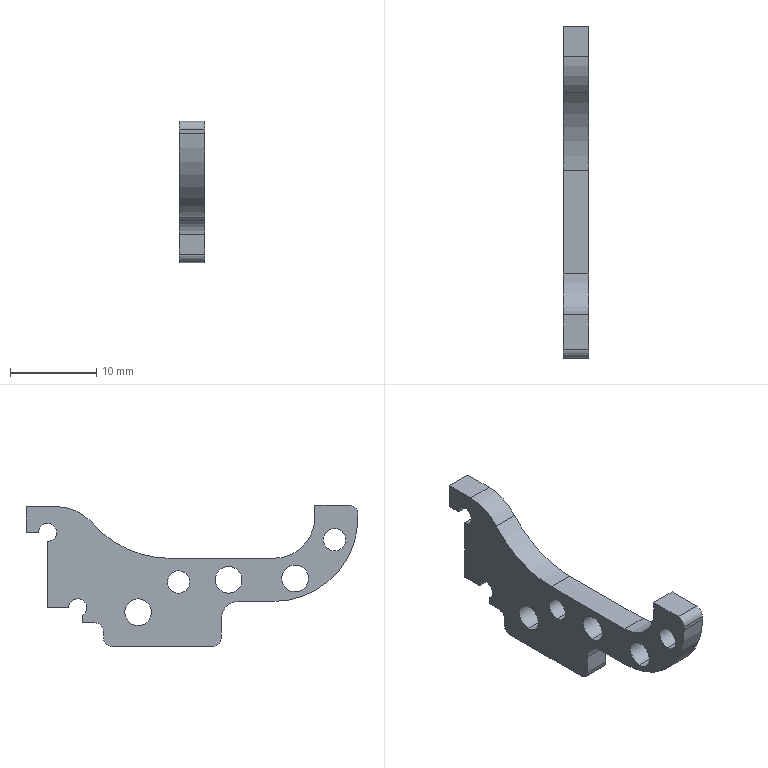Part | SolidWorks | features Fillet 2, Extrusion 1, ICE 1 | 1 solid | 38 faces | box 3 x 38.5 x 16.4 mm | volume 858.003 mm3 | cylinder 21 | plane 17 | commonest cylinder face diameters 3.1 x6 2 x4 2.6 x4 2.1 x2 4 x1 9.5 x1
STEP:
#1=CARTESIAN_POINT('',(3.,5.25,15.2));
#2=VERTEX_POINT('',#1);
#3=CARTESIAN_POINT('',(3.,5.25,18.3));
#4=VERTEX_POINT('',#3);
#5=CARTESIAN_POINT('',(3.,5.25,16.75));
#6=DIRECTION('',(-1.,0.,0.));
#7=DIRECTION('',(0.,0.,-1.));
#8=AXIS2_PLACEMENT_3D('',#5,#6,#7);
#9=CIRCLE('',#8,1.55);
#10=EDGE_CURVE('',#2,#4,#9,.T.);
#11=ORIENTED_EDGE('',*,*,#10,.F.);
#12=CARTESIAN_POINT('',(0.,5.25,15.2));
#13=VERTEX_POINT('',#12);
#14=CARTESIAN_POINT('',(3.,5.25,15.2));
#15=DIRECTION('',(-1.,0.,0.));
#16=VECTOR('',#15,1000.);
#17=LINE('',#14,#16);
#18=EDGE_CURVE('',#2,#13,#17,.T.);
#19=ORIENTED_EDGE('',*,*,#18,.T.);
#20=CARTESIAN_POINT('',(0.,5.25,18.3));
#21=VERTEX_POINT('',#20);
#22=CARTESIAN_POINT('',(0.,5.25,16.75));
#23=DIRECTION('',(-1.,0.,0.));
#24=DIRECTION('',(0.,0.,-1.));
#25=AXIS2_PLACEMENT_3D('',#22,#23,#24);
#26=CIRCLE('',#25,1.55);
#27=EDGE_CURVE('',#13,#21,#26,.T.);
#28=ORIENTED_EDGE('',*,*,#27,.T.);
#29=CARTESIAN_POINT('',(3.,5.25,18.3));
#30=DIRECTION('',(-1.,0.,0.));
#31=VECTOR('',#30,1000.);
#32=LINE('',#29,#31);
#33=EDGE_CURVE('',#4,#21,#32,.T.);
#34=ORIENTED_EDGE('',*,*,#33,.F.);
#35=EDGE_LOOP('',(#11,#19,#28,#34));
#36=FACE_OUTER_BOUND('',#35,.T.);
#37=CARTESIAN_POINT('',(3.,5.25,16.75));
#38=DIRECTION('',(-1.,0.,0.));
#39=DIRECTION('',(0.,0.,1.));
#40=AXIS2_PLACEMENT_3D('',#37,#38,#39);
#41=CYLINDRICAL_SURFACE('',#40,1.55);
#42=ADVANCED_FACE('',(#36),#41,.F.);
#43=CARTESIAN_POINT('',(3.,11.05,17.8));
#44=VERTEX_POINT('',#43);
#45=CARTESIAN_POINT('',(3.,11.05,15.2));
#46=VERTEX_POINT('',#45);
#47=CARTESIAN_POINT('',(3.,11.05,16.5));
#48=DIRECTION('',(1.,0.,0.));
#49=DIRECTION('',(0.,0.,-1.));
#50=AXIS2_PLACEMENT_3D('',#47,#48,#49);
#51=CIRCLE('',#50,1.3);
#52=EDGE_CURVE('',#44,#46,#51,.T.);
#53=ORIENTED_EDGE('',*,*,#52,.T.);
#54=CARTESIAN_POINT('',(0.,11.05,15.2));
#55=VERTEX_POINT('',#54);
#56=CARTESIAN_POINT('',(3.,11.05,15.2));
#57=DIRECTION('',(-1.,0.,0.));
#58=VECTOR('',#57,1000.);
#59=LINE('',#56,#58);
#60=EDGE_CURVE('',#46,#55,#59,.T.);
#61=ORIENTED_EDGE('',*,*,#60,.T.);
#62=CARTESIAN_POINT('',(0.,11.05,17.8));
#63=VERTEX_POINT('',#62);
#64=CARTESIAN_POINT('',(0.,11.05,16.5));
#65=DIRECTION('',(1.,0.,0.));
#66=DIRECTION('',(0.,0.,-1.));
#67=AXIS2_PLACEMENT_3D('',#64,#65,#66);
#68=CIRCLE('',#67,1.3);
#69=EDGE_CURVE('',#63,#55,#68,.T.);
#70=ORIENTED_EDGE('',*,*,#69,.F.);
#71=CARTESIAN_POINT('',(3.,11.05,17.8));
#72=DIRECTION('',(-1.,0.,0.));
#73=VECTOR('',#72,1000.);
#74=LINE('',#71,#73);
#75=EDGE_CURVE('',#44,#63,#74,.T.);
#76=ORIENTED_EDGE('',*,*,#75,.F.);
#77=EDGE_LOOP('',(#53,#61,#70,#76));
#78=FACE_OUTER_BOUND('',#77,.T.);
#79=CARTESIAN_POINT('',(3.,11.05,16.5));
#80=DIRECTION('',(-1.,0.,0.));
#81=DIRECTION('',(0.,0.,1.));
#82=AXIS2_PLACEMENT_3D('',#79,#80,#81);
#83=CYLINDRICAL_SURFACE('',#82,1.3);
#84=ADVANCED_FACE('',(#78),#83,.F.);
#85=CARTESIAN_POINT('',(3.,15.75,14.55));
#86=VERTEX_POINT('',#85);
#87=CARTESIAN_POINT('',(3.,15.75,11.45));
#88=VERTEX_POINT('',#87);
#89=CARTESIAN_POINT('',(3.,15.75,13.));
#90=DIRECTION('',(1.,0.,0.));
#91=DIRECTION('',(0.,0.,-1.));
#92=AXIS2_PLACEMENT_3D('',#89,#90,#91);
#93=CIRCLE('',#92,1.55);
#94=EDGE_CURVE('',#86,#88,#93,.T.);
#95=ORIENTED_EDGE('',*,*,#94,.T.);
#96=CARTESIAN_POINT('',(0.,15.75,11.45));
#97=VERTEX_POINT('',#96);
#98=CARTESIAN_POINT('',(3.,15.75,11.45));
#99=DIRECTION('',(-1.,0.,0.));
#100=VECTOR('',#99,1000.);
#101=LINE('',#98,#100);
#102=EDGE_CURVE('',#88,#97,#101,.T.);
#103=ORIENTED_EDGE('',*,*,#102,.T.);
#104=CARTESIAN_POINT('',(0.,15.75,14.55));
#105=VERTEX_POINT('',#104);
#106=CARTESIAN_POINT('',(0.,15.75,13.));
#107=DIRECTION('',(1.,0.,0.));
#108=DIRECTION('',(0.,0.,-1.));
#109=AXIS2_PLACEMENT_3D('',#106,#107,#108);
#110=CIRCLE('',#109,1.55);
#111=EDGE_CURVE('',#105,#97,#110,.T.);
#112=ORIENTED_EDGE('',*,*,#111,.F.);
#113=CARTESIAN_POINT('',(3.,15.75,14.55));
#114=DIRECTION('',(-1.,0.,0.));
#115=VECTOR('',#114,1000.);
#116=LINE('',#113,#115);
#117=EDGE_CURVE('',#86,#105,#116,.T.);
#118=ORIENTED_EDGE('',*,*,#117,.F.);
#119=EDGE_LOOP('',(#95,#103,#112,#118));
#120=FACE_OUTER_BOUND('',#119,.T.);
#121=CARTESIAN_POINT('',(3.,15.75,13.));
#122=DIRECTION('',(-1.,0.,0.));
#123=DIRECTION('',(0.,0.,1.));
#124=AXIS2_PLACEMENT_3D('',#121,#122,#123);
#125=CYLINDRICAL_SURFACE('',#124,1.55);
#126=ADVANCED_FACE('',(#120),#125,.F.);
#127=CARTESIAN_POINT('',(3.,-7.035,22.7));
#128=VERTEX_POINT('',#127);
#129=CARTESIAN_POINT('',(3.,-7.035,20.1));
#130=VERTEX_POINT('',#129);
#131=CARTESIAN_POINT('',(3.,-7.035,21.4));
#132=DIRECTION('',(1.,0.,0.));
#133=DIRECTION('',(0.,0.,-1.));
#134=AXIS2_PLACEMENT_3D('',#131,#132,#133);
#135=CIRCLE('',#134,1.3);
#136=EDGE_CURVE('',#128,#130,#135,.T.);
#137=ORIENTED_EDGE('',*,*,#136,.T.);
#138=CARTESIAN_POINT('',(0.,-7.035,20.1));
#139=VERTEX_POINT('',#138);
#140=CARTESIAN_POINT('',(3.,-7.035,20.1));
#141=DIRECTION('',(-1.,0.,0.));
#142=VECTOR('',#141,1000.);
#143=LINE('',#140,#142);
#144=EDGE_CURVE('',#130,#139,#143,.T.);
#145=ORIENTED_EDGE('',*,*,#144,.T.);
#146=CARTESIAN_POINT('',(0.,-7.035,22.7));
#147=VERTEX_POINT('',#146);
#148=CARTESIAN_POINT('',(0.,-7.035,21.4));
#149=DIRECTION('',(1.,0.,0.));
#150=DIRECTION('',(0.,0.,-1.));
#151=AXIS2_PLACEMENT_3D('',#148,#149,#150);
#152=CIRCLE('',#151,1.3);
#153=EDGE_CURVE('',#147,#139,#152,.T.);
#154=ORIENTED_EDGE('',*,*,#153,.F.);
#155=CARTESIAN_POINT('',(3.,-7.035,22.7));
#156=DIRECTION('',(-1.,0.,0.));
#157=VECTOR('',#156,1000.);
#158=LINE('',#155,#157);
#159=EDGE_CURVE('',#128,#147,#158,.T.);
#160=ORIENTED_EDGE('',*,*,#159,.F.);
#161=EDGE_LOOP('',(#137,#145,#154,#160));
#162=FACE_OUTER_BOUND('',#161,.T.);
#163=CARTESIAN_POINT('',(3.,-7.035,21.4));
#164=DIRECTION('',(-1.,0.,0.));
#165=DIRECTION('',(0.,0.,1.));
#166=AXIS2_PLACEMENT_3D('',#163,#164,#165);
#167=CYLINDRICAL_SURFACE('',#166,1.3);
#168=ADVANCED_FACE('',(#162),#167,.F.);
#169=CARTESIAN_POINT('',(3.,-2.467,18.467));
#170=VERTEX_POINT('',#169);
#171=CARTESIAN_POINT('',(3.,-2.467,15.367));
#172=VERTEX_POINT('',#171);
#173=CARTESIAN_POINT('',(3.,-2.467,16.917));
#174=DIRECTION('',(1.,0.,0.));
#175=DIRECTION('',(0.,0.,-1.));
#176=AXIS2_PLACEMENT_3D('',#173,#174,#175);
#177=CIRCLE('',#176,1.55);
#178=EDGE_CURVE('',#170,#172,#177,.T.);
#179=ORIENTED_EDGE('',*,*,#178,.T.);
#180=CARTESIAN_POINT('',(0.,-2.467,15.367));
#181=VERTEX_POINT('',#180);
#182=CARTESIAN_POINT('',(3.,-2.467,15.367));
#183=DIRECTION('',(-1.,0.,0.));
#184=VECTOR('',#183,1000.);
#185=LINE('',#182,#184);
#186=EDGE_CURVE('',#172,#181,#185,.T.);
#187=ORIENTED_EDGE('',*,*,#186,.T.);
#188=CARTESIAN_POINT('',(0.,-2.467,18.467));
#189=VERTEX_POINT('',#188);
#190=CARTESIAN_POINT('',(0.,-2.467,16.917));
#191=DIRECTION('',(1.,0.,0.));
#192=DIRECTION('',(0.,0.,-1.));
#193=AXIS2_PLACEMENT_3D('',#190,#191,#192);
#194=CIRCLE('',#193,1.55);
#195=EDGE_CURVE('',#189,#181,#194,.T.);
#196=ORIENTED_EDGE('',*,*,#195,.F.);
#197=CARTESIAN_POINT('',(3.,-2.467,18.467));
#198=DIRECTION('',(-1.,0.,0.));
#199=VECTOR('',#198,1000.);
#200=LINE('',#197,#199);
#201=EDGE_CURVE('',#170,#189,#200,.T.);
#202=ORIENTED_EDGE('',*,*,#201,.F.);
#203=EDGE_LOOP('',(#179,#187,#196,#202));
#204=FACE_OUTER_BOUND('',#203,.T.);
#205=CARTESIAN_POINT('',(3.,-2.467,16.917));
#206=DIRECTION('',(-1.,0.,0.));
#207=DIRECTION('',(0.,0.,1.));
#208=AXIS2_PLACEMENT_3D('',#205,#206,#207);
#209=CYLINDRICAL_SURFACE('',#208,1.55);
#210=ADVANCED_FACE('',(#204),#209,.F.);
#211=CARTESIAN_POINT('',(3.,0.,19.25));
#212=VERTEX_POINT('',#211);
#213=CARTESIAN_POINT('',(3.,12.036,19.25));
#214=VERTEX_POINT('',#213);
#215=CARTESIAN_POINT('',(3.,0.,19.25));
#216=DIRECTION('',(0.,1.,0.));
#217=VECTOR('',#216,1000.);
#218=LINE('',#215,#217);
#219=EDGE_CURVE('',#212,#214,#218,.T.);
#220=ORIENTED_EDGE('',*,*,#219,.T.);
#221=CARTESIAN_POINT('',(0.,12.036,19.25));
#222=VERTEX_POINT('',#221);
#223=CARTESIAN_POINT('',(0.,12.036,19.25));
#224=DIRECTION('',(1.,0.,0.));
#225=VECTOR('',#224,1000.);
#226=LINE('',#223,#225);
#227=EDGE_CURVE('',#222,#214,#226,.T.);
#228=ORIENTED_EDGE('',*,*,#227,.F.);
#229=CARTESIAN_POINT('',(0.,0.,19.25));
#230=VERTEX_POINT('',#229);
#231=CARTESIAN_POINT('',(0.,0.,19.25));
#232=DIRECTION('',(0.,1.,0.));
#233=VECTOR('',#232,1000.);
#234=LINE('',#231,#233);
#235=EDGE_CURVE('',#230,#222,#234,.T.);
#236=ORIENTED_EDGE('',*,*,#235,.F.);
#237=CARTESIAN_POINT('',(3.,0.,19.25));
#238=DIRECTION('',(-1.,0.,0.));
#239=VECTOR('',#238,1000.);
#240=LINE('',#237,#239);
#241=EDGE_CURVE('',#212,#230,#240,.T.);
#242=ORIENTED_EDGE('',*,*,#241,.F.);
#243=EDGE_LOOP('',(#220,#228,#236,#242));
#244=FACE_OUTER_BOUND('',#243,.T.);
#245=CARTESIAN_POINT('',(3.,0.,19.25));
#246=DIRECTION('',(0.,0.,1.));
#247=DIRECTION('',(0.,-1.,0.));
#248=AXIS2_PLACEMENT_3D('',#245,#246,#247);
#249=PLANE('',#248);
#250=ADVANCED_FACE('',(#244),#249,.T.);
#251=CARTESIAN_POINT('',(3.,19.75,10.75));
#252=VERTEX_POINT('',#251);
#253=CARTESIAN_POINT('',(3.,19.75,10.));
#254=VERTEX_POINT('',#253);
#255=CARTESIAN_POINT('',(3.,19.75,0.));
#256=DIRECTION('',(0.,0.,-1.));
#257=VECTOR('',#256,1000.);
#258=LINE('',#255,#257);
#259=EDGE_CURVE('',#252,#254,#258,.T.);
#260=ORIENTED_EDGE('',*,*,#259,.T.);
#261=CARTESIAN_POINT('',(0.,19.75,10.));
#262=VERTEX_POINT('',#261);
#263=CARTESIAN_POINT('',(3.,19.75,10.));
#264=DIRECTION('',(-1.,0.,0.));
#265=VECTOR('',#264,1000.);
#266=LINE('',#263,#265);
#267=EDGE_CURVE('',#254,#262,#266,.T.);
#268=ORIENTED_EDGE('',*,*,#267,.T.);
#269=CARTESIAN_POINT('',(0.,19.75,10.75));
#270=VERTEX_POINT('',#269);
#271=CARTESIAN_POINT('',(0.,19.75,0.));
#272=DIRECTION('',(0.,0.,-1.));
#273=VECTOR('',#272,1000.);
#274=LINE('',#271,#273);
#275=EDGE_CURVE('',#270,#262,#274,.T.);
#276=ORIENTED_EDGE('',*,*,#275,.F.);
#277=CARTESIAN_POINT('',(3.,19.75,10.75));
#278=DIRECTION('',(1.,0.,0.));
#279=VECTOR('',#278,1000.);
#280=LINE('',#277,#279);
#281=EDGE_CURVE('',#270,#252,#280,.T.);
#282=ORIENTED_EDGE('',*,*,#281,.T.);
#283=EDGE_LOOP('',(#260,#268,#276,#282));
#284=FACE_OUTER_BOUND('',#283,.T.);
#285=CARTESIAN_POINT('',(3.,19.75,0.));
#286=DIRECTION('',(0.,1.,0.));
#287=DIRECTION('',(0.,0.,1.));
#288=AXIS2_PLACEMENT_3D('',#285,#286,#287);
#289=PLANE('',#288);
#290=ADVANCED_FACE('',(#284),#289,.T.);
#291=CARTESIAN_POINT('',(0.,-4.75,24.));
#292=VERTEX_POINT('',#291);
#293=CARTESIAN_POINT('',(0.,0.,24.));
#294=DIRECTION('',(1.,0.,0.));
#295=DIRECTION('',(0.,0.,-1.));
#296=AXIS2_PLACEMENT_3D('',#293,#294,#295);
#297=CIRCLE('',#296,4.75);
#298=EDGE_CURVE('',#292,#230,#297,.T.);
#299=ORIENTED_EDGE('',*,*,#298,.F.);
#300=CARTESIAN_POINT('',(3.,-4.75,24.));
#301=VERTEX_POINT('',#300);
#302=CARTESIAN_POINT('',(3.,-4.75,24.));
#303=DIRECTION('',(-1.,0.,0.));
#304=VECTOR('',#303,1000.);
#305=LINE('',#302,#304);
#306=EDGE_CURVE('',#301,#292,#305,.T.);
#307=ORIENTED_EDGE('',*,*,#306,.F.);
#308=CARTESIAN_POINT('',(3.,0.,24.));
#309=DIRECTION('',(1.,0.,0.));
#310=DIRECTION('',(0.,0.,-1.));
#311=AXIS2_PLACEMENT_3D('',#308,#309,#310);
#312=CIRCLE('',#311,4.75);
#313=EDGE_CURVE('',#301,#212,#312,.T.);
#314=ORIENTED_EDGE('',*,*,#313,.T.);
#315=ORIENTED_EDGE('',*,*,#241,.T.);
#316=EDGE_LOOP('',(#299,#307,#314,#315));
#317=FACE_OUTER_BOUND('',#316,.T.);
#318=CARTESIAN_POINT('',(3.,0.,24.));
#319=DIRECTION('',(-1.,0.,0.));
#320=DIRECTION('',(0.,0.,1.));
#321=AXIS2_PLACEMENT_3D('',#318,#319,#320);
#322=CYLINDRICAL_SURFACE('',#321,4.75);
#323=ADVANCED_FACE('',(#317),#322,.F.);
#324=CARTESIAN_POINT('',(0.,-4.75,25.4));
#325=VERTEX_POINT('',#324);
#326=CARTESIAN_POINT('',(0.,-4.75,0.));
#327=DIRECTION('',(0.,0.,1.));
#328=VECTOR('',#327,1000.);
#329=LINE('',#326,#328);
#330=EDGE_CURVE('',#292,#325,#329,.T.);
#331=ORIENTED_EDGE('',*,*,#330,.T.);
#332=CARTESIAN_POINT('',(3.,-4.75,25.4));
#333=VERTEX_POINT('',#332);
#334=CARTESIAN_POINT('',(3.,-4.75,25.4));
#335=DIRECTION('',(-1.,0.,0.));
#336=VECTOR('',#335,1000.);
#337=LINE('',#334,#336);
#338=EDGE_CURVE('',#333,#325,#337,.T.);
#339=ORIENTED_EDGE('',*,*,#338,.F.);
#340=CARTESIAN_POINT('',(3.,-4.75,0.));
#341=DIRECTION('',(0.,0.,1.));
#342=VECTOR('',#341,1000.);
#343=LINE('',#340,#342);
#344=EDGE_CURVE('',#301,#333,#343,.T.);
#345=ORIENTED_EDGE('',*,*,#344,.F.);
#346=ORIENTED_EDGE('',*,*,#306,.T.);
#347=EDGE_LOOP('',(#331,#339,#345,#346));
#348=FACE_OUTER_BOUND('',#347,.T.);
#349=CARTESIAN_POINT('',(3.,-4.75,0.));
#350=DIRECTION('',(0.,-1.,0.));
#351=DIRECTION('',(0.,0.,-1.));
#352=AXIS2_PLACEMENT_3D('',#349,#350,#351);
#353=PLANE('',#352);
#354=ADVANCED_FACE('',(#348),#353,.F.);
#355=CARTESIAN_POINT('',(0.,-8.75,25.4));
#356=VERTEX_POINT('',#355);
#357=CARTESIAN_POINT('',(0.,0.,25.4));
#358=DIRECTION('',(0.,-1.,0.));
#359=VECTOR('',#358,1000.);
#360=LINE('',#357,#359);
#361=EDGE_CURVE('',#325,#356,#360,.T.);
#362=ORIENTED_EDGE('',*,*,#361,.T.);
#363=CARTESIAN_POINT('',(3.,-8.75,25.4));
#364=VERTEX_POINT('',#363);
#365=CARTESIAN_POINT('',(3.,-8.75,25.4));
#366=DIRECTION('',(1.,0.,0.));
#367=VECTOR('',#366,1000.);
#368=LINE('',#365,#367);
#369=EDGE_CURVE('',#356,#364,#368,.T.);
#370=ORIENTED_EDGE('',*,*,#369,.T.);
#371=CARTESIAN_POINT('',(3.,0.,25.4));
#372=DIRECTION('',(0.,-1.,0.));
#373=VECTOR('',#372,1000.);
#374=LINE('',#371,#373);
#375=EDGE_CURVE('',#333,#364,#374,.T.);
#376=ORIENTED_EDGE('',*,*,#375,.F.);
#377=ORIENTED_EDGE('',*,*,#338,.T.);
#378=EDGE_LOOP('',(#362,#370,#376,#377));
#379=FACE_OUTER_BOUND('',#378,.T.);
#380=CARTESIAN_POINT('',(3.,0.,25.4));
#381=DIRECTION('',(0.,0.,-1.));
#382=DIRECTION('',(0.,1.,0.));
#383=AXIS2_PLACEMENT_3D('',#380,#381,#382);
#384=PLANE('',#383);
#385=ADVANCED_FACE('',(#379),#384,.F.);
#386=CARTESIAN_POINT('',(3.,-9.75,24.4));
#387=VERTEX_POINT('',#386);
#388=CARTESIAN_POINT('',(3.,-9.75,24.));
#389=VERTEX_POINT('',#388);
#390=CARTESIAN_POINT('',(3.,-9.75,0.));
#391=DIRECTION('',(0.,0.,-1.));
#392=VECTOR('',#391,1000.);
#393=LINE('',#390,#392);
#394=EDGE_CURVE('',#387,#389,#393,.T.);
#395=ORIENTED_EDGE('',*,*,#394,.F.);
#396=CARTESIAN_POINT('',(0.,-9.75,24.4));
#397=VERTEX_POINT('',#396);
#398=CARTESIAN_POINT('',(3.,-9.75,24.4));
#399=DIRECTION('',(-1.,0.,0.));
#400=VECTOR('',#399,1000.);
#401=LINE('',#398,#400);
#402=EDGE_CURVE('',#387,#397,#401,.T.);
#403=ORIENTED_EDGE('',*,*,#402,.T.);
#404=CARTESIAN_POINT('',(0.,-9.75,24.));
#405=VERTEX_POINT('',#404);
#406=CARTESIAN_POINT('',(0.,-9.75,0.));
#407=DIRECTION('',(0.,0.,-1.));
#408=VECTOR('',#407,1000.);
#409=LINE('',#406,#408);
#410=EDGE_CURVE('',#397,#405,#409,.T.);
#411=ORIENTED_EDGE('',*,*,#410,.T.);
#412=CARTESIAN_POINT('',(3.,-9.75,24.));
#413=DIRECTION('',(-1.,0.,0.));
#414=VECTOR('',#413,1000.);
#415=LINE('',#412,#414);
#416=EDGE_CURVE('',#389,#405,#415,.T.);
#417=ORIENTED_EDGE('',*,*,#416,.F.);
#418=EDGE_LOOP('',(#395,#403,#411,#417));
#419=FACE_OUTER_BOUND('',#418,.T.);
#420=CARTESIAN_POINT('',(3.,-9.75,0.));
#421=DIRECTION('',(0.,1.,0.));
#422=DIRECTION('',(0.,0.,1.));
#423=AXIS2_PLACEMENT_3D('',#420,#421,#422);
#424=PLANE('',#423);
#425=ADVANCED_FACE('',(#419),#424,.F.);
#426=CARTESIAN_POINT('',(0.,0.,14.25));
#427=VERTEX_POINT('',#426);
#428=CARTESIAN_POINT('',(0.,0.,24.));
#429=DIRECTION('',(1.,0.,0.));
#430=DIRECTION('',(0.,0.,-1.));
#431=AXIS2_PLACEMENT_3D('',#428,#429,#430);
#432=CIRCLE('',#431,9.75);
#433=EDGE_CURVE('',#405,#427,#432,.T.);
#434=ORIENTED_EDGE('',*,*,#433,.T.);
#435=CARTESIAN_POINT('',(3.,0.,14.25));
#436=VERTEX_POINT('',#435);
#437=CARTESIAN_POINT('',(3.,0.,14.25));
#438=DIRECTION('',(-1.,0.,0.));
#439=VECTOR('',#438,1000.);
#440=LINE('',#437,#439);
#441=EDGE_CURVE('',#436,#427,#440,.T.);
#442=ORIENTED_EDGE('',*,*,#441,.F.);
#443=CARTESIAN_POINT('',(3.,0.,24.));
#444=DIRECTION('',(1.,0.,0.));
#445=DIRECTION('',(0.,0.,-1.));
#446=AXIS2_PLACEMENT_3D('',#443,#444,#445);
#447=CIRCLE('',#446,9.75);
#448=EDGE_CURVE('',#389,#436,#447,.T.);
#449=ORIENTED_EDGE('',*,*,#448,.F.);
#450=ORIENTED_EDGE('',*,*,#416,.T.);
#451=EDGE_LOOP('',(#434,#442,#449,#450));
#452=FACE_OUTER_BOUND('',#451,.T.);
#453=CARTESIAN_POINT('',(3.,0.,24.));
#454=DIRECTION('',(-1.,0.,0.));
#455=DIRECTION('',(0.,0.,1.));
#456=AXIS2_PLACEMENT_3D('',#453,#454,#455);
#457=CYLINDRICAL_SURFACE('',#456,9.75);
#458=ADVANCED_FACE('',(#452),#457,.T.);
#459=CARTESIAN_POINT('',(0.,4.116,14.25));
#460=VERTEX_POINT('',#459);
#461=CARTESIAN_POINT('',(0.,0.,14.25));
#462=DIRECTION('',(0.,1.,0.));
#463=VECTOR('',#462,1000.);
#464=LINE('',#461,#463);
#465=EDGE_CURVE('',#427,#460,#464,.T.);
#466=ORIENTED_EDGE('',*,*,#465,.T.);
#467=CARTESIAN_POINT('',(3.,4.116,14.25));
#468=VERTEX_POINT('',#467);
#469=CARTESIAN_POINT('',(3.,4.116,14.25));
#470=DIRECTION('',(1.,0.,0.));
#471=VECTOR('',#470,1000.);
#472=LINE('',#469,#471);
#473=EDGE_CURVE('',#460,#468,#472,.T.);
#474=ORIENTED_EDGE('',*,*,#473,.T.);
#475=CARTESIAN_POINT('',(3.,0.,14.25));
#476=DIRECTION('',(0.,1.,0.));
#477=VECTOR('',#476,1000.);
#478=LINE('',#475,#477);
#479=EDGE_CURVE('',#436,#468,#478,.T.);
#480=ORIENTED_EDGE('',*,*,#479,.F.);
#481=ORIENTED_EDGE('',*,*,#441,.T.);
#482=EDGE_LOOP('',(#466,#474,#480,#481));
#483=FACE_OUTER_BOUND('',#482,.T.);
#484=CARTESIAN_POINT('',(3.,0.,14.25));
#485=DIRECTION('',(0.,0.,1.));
#486=DIRECTION('',(1.,0.,0.));
#487=AXIS2_PLACEMENT_3D('',#484,#485,#486);
#488=PLANE('',#487);
#489=ADVANCED_FACE('',(#483),#488,.F.);
#490=ORIENTED_EDGE('',*,*,#186,.F.);
#491=CARTESIAN_POINT('',(3.,-2.467,16.917));
#492=DIRECTION('',(1.,0.,0.));
#493=DIRECTION('',(0.,0.,-1.));
#494=AXIS2_PLACEMENT_3D('',#491,#492,#493);
#495=CIRCLE('',#494,1.55);
#496=EDGE_CURVE('',#172,#170,#495,.T.);
#497=ORIENTED_EDGE('',*,*,#496,.T.);
#498=ORIENTED_EDGE('',*,*,#201,.T.);
#499=CARTESIAN_POINT('',(0.,-2.467,16.917));
#500=DIRECTION('',(1.,0.,0.));
#501=DIRECTION('',(0.,0.,-1.));
#502=AXIS2_PLACEMENT_3D('',#499,#500,#501);
#503=CIRCLE('',#502,1.55);
#504=EDGE_CURVE('',#181,#189,#503,.T.);
#505=ORIENTED_EDGE('',*,*,#504,.F.);
#506=EDGE_LOOP('',(#490,#497,#498,#505));
#507=FACE_OUTER_BOUND('',#506,.T.);
#508=CARTESIAN_POINT('',(3.,-2.467,16.917));
#509=DIRECTION('',(-1.,0.,0.));
#510=DIRECTION('',(0.,0.,1.));
#511=AXIS2_PLACEMENT_3D('',#508,#509,#510);
#512=CYLINDRICAL_SURFACE('',#511,1.55);
#513=ADVANCED_FACE('',(#507),#512,.F.);
#514=ORIENTED_EDGE('',*,*,#144,.F.);
#515=CARTESIAN_POINT('',(3.,-7.035,21.4));
#516=DIRECTION('',(1.,0.,0.));
#517=DIRECTION('',(0.,0.,-1.));
#518=AXIS2_PLACEMENT_3D('',#515,#516,#517);
#519=CIRCLE('',#518,1.3);
#520=EDGE_CURVE('',#130,#128,#519,.T.);
#521=ORIENTED_EDGE('',*,*,#520,.T.);
#522=ORIENTED_EDGE('',*,*,#159,.T.);
#523=CARTESIAN_POINT('',(0.,-7.035,21.4));
#524=DIRECTION('',(1.,0.,0.));
#525=DIRECTION('',(0.,0.,-1.));
#526=AXIS2_PLACEMENT_3D('',#523,#524,#525);
#527=CIRCLE('',#526,1.3);
#528=EDGE_CURVE('',#139,#147,#527,.T.);
#529=ORIENTED_EDGE('',*,*,#528,.F.);
#530=EDGE_LOOP('',(#514,#521,#522,#529));
#531=FACE_OUTER_BOUND('',#530,.T.);
#532=CARTESIAN_POINT('',(3.,-7.035,21.4));
#533=DIRECTION('',(-1.,0.,0.));
#534=DIRECTION('',(0.,0.,1.));
#535=AXIS2_PLACEMENT_3D('',#532,#533,#534);
#536=CYLINDRICAL_SURFACE('',#535,1.3);
#537=ADVANCED_FACE('',(#531),#536,.F.);
#538=ORIENTED_EDGE('',*,*,#102,.F.);
#539=CARTESIAN_POINT('',(3.,15.75,13.));
#540=DIRECTION('',(1.,0.,0.));
#541=DIRECTION('',(0.,0.,-1.));
#542=AXIS2_PLACEMENT_3D('',#539,#540,#541);
#543=CIRCLE('',#542,1.55);
#544=EDGE_CURVE('',#88,#86,#543,.T.);
#545=ORIENTED_EDGE('',*,*,#544,.T.);
#546=ORIENTED_EDGE('',*,*,#117,.T.);
#547=CARTESIAN_POINT('',(0.,15.75,13.));
#548=DIRECTION('',(1.,0.,0.));
#549=DIRECTION('',(0.,0.,-1.));
#550=AXIS2_PLACEMENT_3D('',#547,#548,#549);
#551=CIRCLE('',#550,1.55);
#552=EDGE_CURVE('',#97,#105,#551,.T.);
#553=ORIENTED_EDGE('',*,*,#552,.F.);
#554=EDGE_LOOP('',(#538,#545,#546,#553));
#555=FACE_OUTER_BOUND('',#554,.T.);
#556=CARTESIAN_POINT('',(3.,15.75,13.));
#557=DIRECTION('',(-1.,0.,0.));
#558=DIRECTION('',(0.,0.,1.));
#559=AXIS2_PLACEMENT_3D('',#556,#557,#558);
#560=CYLINDRICAL_SURFACE('',#559,1.55);
#561=ADVANCED_FACE('',(#555),#560,.F.);
#562=ORIENTED_EDGE('',*,*,#60,.F.);
#563=CARTESIAN_POINT('',(3.,11.05,16.5));
#564=DIRECTION('',(1.,0.,0.));
#565=DIRECTION('',(0.,0.,-1.));
#566=AXIS2_PLACEMENT_3D('',#563,#564,#565);
#567=CIRCLE('',#566,1.3);
#568=EDGE_CURVE('',#46,#44,#567,.T.);
#569=ORIENTED_EDGE('',*,*,#568,.T.);
#570=ORIENTED_EDGE('',*,*,#75,.T.);
#571=CARTESIAN_POINT('',(0.,11.05,16.5));
#572=DIRECTION('',(1.,0.,0.));
#573=DIRECTION('',(0.,0.,-1.));
#574=AXIS2_PLACEMENT_3D('',#571,#572,#573);
#575=CIRCLE('',#574,1.3);
#576=EDGE_CURVE('',#55,#63,#575,.T.);
#577=ORIENTED_EDGE('',*,*,#576,.F.);
#578=EDGE_LOOP('',(#562,#569,#570,#577));
#579=FACE_OUTER_BOUND('',#578,.T.);
#580=CARTESIAN_POINT('',(3.,11.05,16.5));
#581=DIRECTION('',(-1.,0.,0.));
#582=DIRECTION('',(0.,0.,1.));
#583=AXIS2_PLACEMENT_3D('',#580,#581,#582);
#584=CYLINDRICAL_SURFACE('',#583,1.3);
#585=ADVANCED_FACE('',(#579),#584,.F.);
#586=CARTESIAN_POINT('',(0.,6.116,12.25));
#587=VERTEX_POINT('',#586);
#588=CARTESIAN_POINT('',(0.,6.116,10.));
#589=VERTEX_POINT('',#588);
#590=CARTESIAN_POINT('',(0.,6.116,0.));
#591=DIRECTION('',(0.,0.,-1.));
#592=VECTOR('',#591,1000.);
#593=LINE('',#590,#592);
#594=EDGE_CURVE('',#587,#589,#593,.T.);
#595=ORIENTED_EDGE('',*,*,#594,.T.);
#596=CARTESIAN_POINT('',(3.,6.116,10.));
#597=VERTEX_POINT('',#596);
#598=CARTESIAN_POINT('',(3.,6.116,10.));
#599=DIRECTION('',(1.,0.,0.));
#600=VECTOR('',#599,1000.);
#601=LINE('',#598,#600);
#602=EDGE_CURVE('',#589,#597,#601,.T.);
#603=ORIENTED_EDGE('',*,*,#602,.T.);
#604=CARTESIAN_POINT('',(3.,6.116,12.25));
#605=VERTEX_POINT('',#604);
#606=CARTESIAN_POINT('',(3.,6.116,0.));
#607=DIRECTION('',(0.,0.,-1.));
#608=VECTOR('',#607,1000.);
#609=LINE('',#606,#608);
#610=EDGE_CURVE('',#605,#597,#609,.T.);
#611=ORIENTED_EDGE('',*,*,#610,.F.);
#612=CARTESIAN_POINT('',(0.,6.116,12.25));
#613=DIRECTION('',(-1.,0.,0.));
#614=VECTOR('',#613,1000.);
#615=LINE('',#612,#614);
#616=EDGE_CURVE('',#605,#587,#615,.T.);
#617=ORIENTED_EDGE('',*,*,#616,.T.);
#618=EDGE_LOOP('',(#595,#603,#611,#617));
#619=FACE_OUTER_BOUND('',#618,.T.);
#620=CARTESIAN_POINT('',(3.,6.116,0.));
#621=DIRECTION('',(0.,1.,0.));
#622=DIRECTION('',(0.,0.,1.));
#623=AXIS2_PLACEMENT_3D('',#620,#621,#622);
#624=PLANE('',#623);
#625=ADVANCED_FACE('',(#619),#624,.F.);
#626=ORIENTED_EDGE('',*,*,#18,.F.);
#627=CARTESIAN_POINT('',(3.,5.25,16.75));
#628=DIRECTION('',(-1.,0.,0.));
#629=DIRECTION('',(0.,0.,-1.));
#630=AXIS2_PLACEMENT_3D('',#627,#628,#629);
#631=CIRCLE('',#630,1.55);
#632=EDGE_CURVE('',#4,#2,#631,.T.);
#633=ORIENTED_EDGE('',*,*,#632,.F.);
#634=ORIENTED_EDGE('',*,*,#33,.T.);
#635=CARTESIAN_POINT('',(0.,5.25,16.75));
#636=DIRECTION('',(-1.,0.,0.));
#637=DIRECTION('',(0.,0.,-1.));
#638=AXIS2_PLACEMENT_3D('',#635,#636,#637);
#639=CIRCLE('',#638,1.55);
#640=EDGE_CURVE('',#21,#13,#639,.T.);
#641=ORIENTED_EDGE('',*,*,#640,.T.);
#642=EDGE_LOOP('',(#626,#633,#634,#641));
#643=FACE_OUTER_BOUND('',#642,.T.);
#644=CARTESIAN_POINT('',(3.,5.25,16.75));
#645=DIRECTION('',(-1.,0.,0.));
#646=DIRECTION('',(0.,0.,1.));
#647=AXIS2_PLACEMENT_3D('',#644,#645,#646);
#648=CYLINDRICAL_SURFACE('',#647,1.55);
#649=ADVANCED_FACE('',(#643),#648,.F.);
#650=CARTESIAN_POINT('',(3.,7.116,9.));
#651=VERTEX_POINT('',#650);
#652=CARTESIAN_POINT('',(3.,18.75,9.));
#653=VERTEX_POINT('',#652);
#654=CARTESIAN_POINT('',(3.,6.116,9.));
#655=DIRECTION('',(0.,1.,0.));
#656=VECTOR('',#655,1000.);
#657=LINE('',#654,#656);
#658=EDGE_CURVE('',#651,#653,#657,.T.);
#659=ORIENTED_EDGE('',*,*,#658,.T.);
#660=CARTESIAN_POINT('',(3.,18.75,10.));
#661=DIRECTION('',(1.,0.,0.));
#662=DIRECTION('',(0.,0.,-1.));
#663=AXIS2_PLACEMENT_3D('',#660,#661,#662);
#664=CIRCLE('',#663,1.);
#665=EDGE_CURVE('',#653,#254,#664,.T.);
#666=ORIENTED_EDGE('',*,*,#665,.T.);
#667=ORIENTED_EDGE('',*,*,#259,.F.);
#668=CARTESIAN_POINT('',(3.,20.75,11.75));
#669=VERTEX_POINT('',#668);
#670=CARTESIAN_POINT('',(3.,20.75,10.75));
#671=DIRECTION('',(-1.,0.,0.));
#672=DIRECTION('',(0.,0.,-1.));
#673=AXIS2_PLACEMENT_3D('',#670,#671,#672);
#674=CIRCLE('',#673,1.);
#675=EDGE_CURVE('',#252,#669,#674,.T.);
#676=ORIENTED_EDGE('',*,*,#675,.T.);
#677=CARTESIAN_POINT('',(3.,22.25,11.75));
#678=VERTEX_POINT('',#677);
#679=CARTESIAN_POINT('',(3.,19.75,11.75));
#680=DIRECTION('',(0.,1.,0.));
#681=VECTOR('',#680,1000.);
#682=LINE('',#679,#681);
#683=EDGE_CURVE('',#669,#678,#682,.T.);
#684=ORIENTED_EDGE('',*,*,#683,.T.);
#685=CARTESIAN_POINT('',(3.,22.25,12.577));
#686=VERTEX_POINT('',#685);
#687=CARTESIAN_POINT('',(3.,22.25,11.75));
#688=DIRECTION('',(0.,0.,1.));
#689=VECTOR('',#688,1000.);
#690=LINE('',#687,#689);
#691=EDGE_CURVE('',#678,#686,#690,.T.);
#692=ORIENTED_EDGE('',*,*,#691,.T.);
#693=CARTESIAN_POINT('',(3.,23.8,13.5));
#694=VERTEX_POINT('',#693);
#695=CARTESIAN_POINT('',(3.,22.75,13.5));
#696=DIRECTION('',(-1.,0.,0.));
#697=DIRECTION('',(0.,0.,-1.));
#698=AXIS2_PLACEMENT_3D('',#695,#696,#697);
#699=CIRCLE('',#698,1.05);
#700=EDGE_CURVE('',#686,#694,#699,.T.);
#701=ORIENTED_EDGE('',*,*,#700,.T.);
#702=CARTESIAN_POINT('',(3.,26.25,13.5));
#703=VERTEX_POINT('',#702);
#704=CARTESIAN_POINT('',(3.,23.8,13.5));
#705=DIRECTION('',(0.,1.,0.));
#706=VECTOR('',#705,1000.);
#707=LINE('',#704,#706);
#708=EDGE_CURVE('',#694,#703,#707,.T.);
#709=ORIENTED_EDGE('',*,*,#708,.T.);
#710=CARTESIAN_POINT('',(3.,26.25,21.2));
#711=VERTEX_POINT('',#710);
#712=CARTESIAN_POINT('',(3.,26.25,13.5));
#713=DIRECTION('',(0.,0.,1.));
#714=VECTOR('',#713,1000.);
#715=LINE('',#712,#714);
#716=EDGE_CURVE('',#703,#711,#715,.T.);
#717=ORIENTED_EDGE('',*,*,#716,.T.);
#718=CARTESIAN_POINT('',(3.,27.3,22.25));
#719=VERTEX_POINT('',#718);
#720=CARTESIAN_POINT('',(3.,26.25,22.25));
#721=DIRECTION('',(-1.,0.,0.));
#722=DIRECTION('',(0.,0.,-1.));
#723=AXIS2_PLACEMENT_3D('',#720,#721,#722);
#724=CIRCLE('',#723,1.05);
#725=EDGE_CURVE('',#711,#719,#724,.T.);
#726=ORIENTED_EDGE('',*,*,#725,.T.);
#727=CARTESIAN_POINT('',(3.,28.75,22.25));
#728=VERTEX_POINT('',#727);
#729=CARTESIAN_POINT('',(3.,27.3,22.25));
#730=DIRECTION('',(0.,1.,0.));
#731=VECTOR('',#730,1000.);
#732=LINE('',#729,#731);
#733=EDGE_CURVE('',#719,#728,#732,.T.);
#734=ORIENTED_EDGE('',*,*,#733,.T.);
#735=CARTESIAN_POINT('',(3.,28.75,25.25));
#736=VERTEX_POINT('',#735);
#737=CARTESIAN_POINT('',(3.,28.75,22.25));
#738=DIRECTION('',(0.,0.,1.));
#739=VECTOR('',#738,1000.);
#740=LINE('',#737,#739);
#741=EDGE_CURVE('',#728,#736,#740,.T.);
#742=ORIENTED_EDGE('',*,*,#741,.T.);
#743=CARTESIAN_POINT('',(3.,25.25,25.25));
#744=VERTEX_POINT('',#743);
#745=CARTESIAN_POINT('',(3.,28.75,25.25));
#746=DIRECTION('',(0.,-1.,0.));
#747=VECTOR('',#746,1000.);
#748=LINE('',#745,#747);
#749=EDGE_CURVE('',#736,#744,#748,.T.);
#750=ORIENTED_EDGE('',*,*,#749,.T.);
#751=CARTESIAN_POINT('',(3.,21.071,23.353));
#752=VERTEX_POINT('',#751);
#753=CARTESIAN_POINT('',(3.,25.25,19.7));
#754=DIRECTION('',(1.,0.,0.));
#755=DIRECTION('',(0.,0.,-1.));
#756=AXIS2_PLACEMENT_3D('',#753,#754,#755);
#757=CIRCLE('',#756,5.55);
#758=EDGE_CURVE('',#744,#752,#757,.T.);
#759=ORIENTED_EDGE('',*,*,#758,.T.);
#760=CARTESIAN_POINT('',(3.,12.036,31.25));
#761=DIRECTION('',(-1.,0.,0.));
#762=DIRECTION('',(0.,0.,-1.));
#763=AXIS2_PLACEMENT_3D('',#760,#761,#762);
#764=CIRCLE('',#763,12.);
#765=EDGE_CURVE('',#752,#214,#764,.T.);
#766=ORIENTED_EDGE('',*,*,#765,.T.);
#767=ORIENTED_EDGE('',*,*,#219,.F.);
#768=ORIENTED_EDGE('',*,*,#313,.F.);
#769=ORIENTED_EDGE('',*,*,#344,.T.);
#770=ORIENTED_EDGE('',*,*,#375,.T.);
#771=CARTESIAN_POINT('',(3.,-8.75,24.4));
#772=DIRECTION('',(1.,0.,0.));
#773=DIRECTION('',(0.,0.,-1.));
#774=AXIS2_PLACEMENT_3D('',#771,#772,#773);
#775=CIRCLE('',#774,1.);
#776=EDGE_CURVE('',#364,#387,#775,.T.);
#777=ORIENTED_EDGE('',*,*,#776,.T.);
#778=ORIENTED_EDGE('',*,*,#394,.T.);
#779=ORIENTED_EDGE('',*,*,#448,.T.);
#780=ORIENTED_EDGE('',*,*,#479,.T.);
#781=CARTESIAN_POINT('',(3.,4.116,12.25));
#782=DIRECTION('',(-1.,0.,0.));
#783=DIRECTION('',(0.,0.,-1.));
#784=AXIS2_PLACEMENT_3D('',#781,#782,#783);
#785=CIRCLE('',#784,2.);
#786=EDGE_CURVE('',#468,#605,#785,.T.);
#787=ORIENTED_EDGE('',*,*,#786,.T.);
#788=ORIENTED_EDGE('',*,*,#610,.T.);
#789=CARTESIAN_POINT('',(3.,7.116,10.));
#790=DIRECTION('',(1.,0.,0.));
#791=DIRECTION('',(0.,0.,-1.));
#792=AXIS2_PLACEMENT_3D('',#789,#790,#791);
#793=CIRCLE('',#792,1.);
#794=EDGE_CURVE('',#597,#651,#793,.T.);
#795=ORIENTED_EDGE('',*,*,#794,.T.);
#796=EDGE_LOOP('',(#659,#666,#667,#676,#684,#692,#701,#709,#717,#726,#734,#742,#750,#759,#766,#767,#768,#769,#770,#777,#778,#779,#780,#787,#788,#795));
#797=FACE_OUTER_BOUND('',#796,.T.);
#798=ORIENTED_EDGE('',*,*,#52,.F.);
#799=ORIENTED_EDGE('',*,*,#568,.F.);
#800=EDGE_LOOP('',(#798,#799));
#801=FACE_BOUND('',#800,.T.);
#802=ORIENTED_EDGE('',*,*,#94,.F.);
#803=ORIENTED_EDGE('',*,*,#544,.F.);
#804=EDGE_LOOP('',(#802,#803));
#805=FACE_BOUND('',#804,.T.);
#806=ORIENTED_EDGE('',*,*,#136,.F.);
#807=ORIENTED_EDGE('',*,*,#520,.F.);
#808=EDGE_LOOP('',(#806,#807));
#809=FACE_BOUND('',#808,.T.);
#810=ORIENTED_EDGE('',*,*,#178,.F.);
#811=ORIENTED_EDGE('',*,*,#496,.F.);
#812=EDGE_LOOP('',(#810,#811));
#813=FACE_BOUND('',#812,.T.);
#814=ORIENTED_EDGE('',*,*,#632,.T.);
#815=ORIENTED_EDGE('',*,*,#10,.T.);
#816=EDGE_LOOP('',(#814,#815));
#817=FACE_BOUND('',#816,.T.);
#818=CARTESIAN_POINT('',(3.,0.,0.));
#819=DIRECTION('',(1.,0.,0.));
#820=DIRECTION('',(0.,0.,-1.));
#821=AXIS2_PLACEMENT_3D('',#818,#819,#820);
#822=PLANE('',#821);
#823=ADVANCED_FACE('',(#797,#801,#805,#809,#813,#817),#822,.T.);
#824=ORIENTED_EDGE('',*,*,#275,.T.);
#825=CARTESIAN_POINT('',(0.,18.75,9.));
#826=VERTEX_POINT('',#825);
#827=CARTESIAN_POINT('',(0.,18.75,10.));
#828=DIRECTION('',(-1.,0.,0.));
#829=DIRECTION('',(0.,0.,-1.));
#830=AXIS2_PLACEMENT_3D('',#827,#828,#829);
#831=CIRCLE('',#830,1.);
#832=EDGE_CURVE('',#262,#826,#831,.T.);
#833=ORIENTED_EDGE('',*,*,#832,.T.);
#834=CARTESIAN_POINT('',(0.,7.116,9.));
#835=VERTEX_POINT('',#834);
#836=CARTESIAN_POINT('',(0.,6.116,9.));
#837=DIRECTION('',(0.,1.,0.));
#838=VECTOR('',#837,1000.);
#839=LINE('',#836,#838);
#840=EDGE_CURVE('',#835,#826,#839,.T.);
#841=ORIENTED_EDGE('',*,*,#840,.F.);
#842=CARTESIAN_POINT('',(0.,7.116,10.));
#843=DIRECTION('',(-1.,0.,0.));
#844=DIRECTION('',(0.,0.,-1.));
#845=AXIS2_PLACEMENT_3D('',#842,#843,#844);
#846=CIRCLE('',#845,1.);
#847=EDGE_CURVE('',#835,#589,#846,.T.);
#848=ORIENTED_EDGE('',*,*,#847,.T.);
#849=ORIENTED_EDGE('',*,*,#594,.F.);
#850=CARTESIAN_POINT('',(0.,4.116,12.25));
#851=DIRECTION('',(1.,0.,0.));
#852=DIRECTION('',(0.,0.,-1.));
#853=AXIS2_PLACEMENT_3D('',#850,#851,#852);
#854=CIRCLE('',#853,2.);
#855=EDGE_CURVE('',#587,#460,#854,.T.);
#856=ORIENTED_EDGE('',*,*,#855,.T.);
#857=ORIENTED_EDGE('',*,*,#465,.F.);
#858=ORIENTED_EDGE('',*,*,#433,.F.);
#859=ORIENTED_EDGE('',*,*,#410,.F.);
#860=CARTESIAN_POINT('',(0.,-8.75,24.4));
#861=DIRECTION('',(-1.,0.,0.));
#862=DIRECTION('',(0.,0.,-1.));
#863=AXIS2_PLACEMENT_3D('',#860,#861,#862);
#864=CIRCLE('',#863,1.);
#865=EDGE_CURVE('',#397,#356,#864,.T.);
#866=ORIENTED_EDGE('',*,*,#865,.T.);
#867=ORIENTED_EDGE('',*,*,#361,.F.);
#868=ORIENTED_EDGE('',*,*,#330,.F.);
#869=ORIENTED_EDGE('',*,*,#298,.T.);
#870=ORIENTED_EDGE('',*,*,#235,.T.);
#871=CARTESIAN_POINT('',(0.,21.071,23.353));
#872=VERTEX_POINT('',#871);
#873=CARTESIAN_POINT('',(0.,12.036,31.25));
#874=DIRECTION('',(-1.,0.,0.));
#875=DIRECTION('',(0.,0.,-1.));
#876=AXIS2_PLACEMENT_3D('',#873,#874,#875);
#877=CIRCLE('',#876,12.);
#878=EDGE_CURVE('',#872,#222,#877,.T.);
#879=ORIENTED_EDGE('',*,*,#878,.F.);
#880=CARTESIAN_POINT('',(0.,25.25,25.25));
#881=VERTEX_POINT('',#880);
#882=CARTESIAN_POINT('',(0.,25.25,19.7));
#883=DIRECTION('',(1.,0.,0.));
#884=DIRECTION('',(0.,0.,-1.));
#885=AXIS2_PLACEMENT_3D('',#882,#883,#884);
#886=CIRCLE('',#885,5.55);
#887=EDGE_CURVE('',#881,#872,#886,.T.);
#888=ORIENTED_EDGE('',*,*,#887,.F.);
#889=CARTESIAN_POINT('',(0.,28.75,25.25));
#890=VERTEX_POINT('',#889);
#891=CARTESIAN_POINT('',(0.,28.75,25.25));
#892=DIRECTION('',(0.,-1.,0.));
#893=VECTOR('',#892,1000.);
#894=LINE('',#891,#893);
#895=EDGE_CURVE('',#890,#881,#894,.T.);
#896=ORIENTED_EDGE('',*,*,#895,.F.);
#897=CARTESIAN_POINT('',(0.,28.75,22.25));
#898=VERTEX_POINT('',#897);
#899=CARTESIAN_POINT('',(0.,28.75,22.25));
#900=DIRECTION('',(0.,0.,1.));
#901=VECTOR('',#900,1000.);
#902=LINE('',#899,#901);
#903=EDGE_CURVE('',#898,#890,#902,.T.);
#904=ORIENTED_EDGE('',*,*,#903,.F.);
#905=CARTESIAN_POINT('',(0.,27.3,22.25));
#906=VERTEX_POINT('',#905);
#907=CARTESIAN_POINT('',(0.,27.3,22.25));
#908=DIRECTION('',(0.,1.,0.));
#909=VECTOR('',#908,1000.);
#910=LINE('',#907,#909);
#911=EDGE_CURVE('',#906,#898,#910,.T.);
#912=ORIENTED_EDGE('',*,*,#911,.F.);
#913=CARTESIAN_POINT('',(0.,26.25,21.2));
#914=VERTEX_POINT('',#913);
#915=CARTESIAN_POINT('',(0.,26.25,22.25));
#916=DIRECTION('',(-1.,0.,0.));
#917=DIRECTION('',(0.,0.,-1.));
#918=AXIS2_PLACEMENT_3D('',#915,#916,#917);
#919=CIRCLE('',#918,1.05);
#920=EDGE_CURVE('',#914,#906,#919,.T.);
#921=ORIENTED_EDGE('',*,*,#920,.F.);
#922=CARTESIAN_POINT('',(0.,26.25,13.5));
#923=VERTEX_POINT('',#922);
#924=CARTESIAN_POINT('',(0.,26.25,13.5));
#925=DIRECTION('',(0.,0.,1.));
#926=VECTOR('',#925,1000.);
#927=LINE('',#924,#926);
#928=EDGE_CURVE('',#923,#914,#927,.T.);
#929=ORIENTED_EDGE('',*,*,#928,.F.);
#930=CARTESIAN_POINT('',(0.,23.8,13.5));
#931=VERTEX_POINT('',#930);
#932=CARTESIAN_POINT('',(0.,23.8,13.5));
#933=DIRECTION('',(0.,1.,0.));
#934=VECTOR('',#933,1000.);
#935=LINE('',#932,#934);
#936=EDGE_CURVE('',#931,#923,#935,.T.);
#937=ORIENTED_EDGE('',*,*,#936,.F.);
#938=CARTESIAN_POINT('',(0.,22.25,12.577));
#939=VERTEX_POINT('',#938);
#940=CARTESIAN_POINT('',(0.,22.75,13.5));
#941=DIRECTION('',(-1.,0.,0.));
#942=DIRECTION('',(0.,0.,-1.));
#943=AXIS2_PLACEMENT_3D('',#940,#941,#942);
#944=CIRCLE('',#943,1.05);
#945=EDGE_CURVE('',#939,#931,#944,.T.);
#946=ORIENTED_EDGE('',*,*,#945,.F.);
#947=CARTESIAN_POINT('',(0.,22.25,11.75));
#948=VERTEX_POINT('',#947);
#949=CARTESIAN_POINT('',(0.,22.25,11.75));
#950=DIRECTION('',(0.,0.,1.));
#951=VECTOR('',#950,1000.);
#952=LINE('',#949,#951);
#953=EDGE_CURVE('',#948,#939,#952,.T.);
#954=ORIENTED_EDGE('',*,*,#953,.F.);
#955=CARTESIAN_POINT('',(0.,20.75,11.75));
#956=VERTEX_POINT('',#955);
#957=CARTESIAN_POINT('',(0.,19.75,11.75));
#958=DIRECTION('',(0.,1.,0.));
#959=VECTOR('',#958,1000.);
#960=LINE('',#957,#959);
#961=EDGE_CURVE('',#956,#948,#960,.T.);
#962=ORIENTED_EDGE('',*,*,#961,.F.);
#963=CARTESIAN_POINT('',(0.,20.75,10.75));
#964=DIRECTION('',(1.,0.,0.));
#965=DIRECTION('',(0.,0.,-1.));
#966=AXIS2_PLACEMENT_3D('',#963,#964,#965);
#967=CIRCLE('',#966,1.);
#968=EDGE_CURVE('',#956,#270,#967,.T.);
#969=ORIENTED_EDGE('',*,*,#968,.T.);
#970=EDGE_LOOP('',(#824,#833,#841,#848,#849,#856,#857,#858,#859,#866,#867,#868,#869,#870,#879,#888,#896,#904,#912,#921,#929,#937,#946,#954,#962,#969));
#971=FACE_OUTER_BOUND('',#970,.T.);
#972=ORIENTED_EDGE('',*,*,#69,.T.);
#973=ORIENTED_EDGE('',*,*,#576,.T.);
#974=EDGE_LOOP('',(#972,#973));
#975=FACE_BOUND('',#974,.T.);
#976=ORIENTED_EDGE('',*,*,#111,.T.);
#977=ORIENTED_EDGE('',*,*,#552,.T.);
#978=EDGE_LOOP('',(#976,#977));
#979=FACE_BOUND('',#978,.T.);
#980=ORIENTED_EDGE('',*,*,#153,.T.);
#981=ORIENTED_EDGE('',*,*,#528,.T.);
#982=EDGE_LOOP('',(#980,#981));
#983=FACE_BOUND('',#982,.T.);
#984=ORIENTED_EDGE('',*,*,#195,.T.);
#985=ORIENTED_EDGE('',*,*,#504,.T.);
#986=EDGE_LOOP('',(#984,#985));
#987=FACE_BOUND('',#986,.T.);
#988=ORIENTED_EDGE('',*,*,#640,.F.);
#989=ORIENTED_EDGE('',*,*,#27,.F.);
#990=EDGE_LOOP('',(#988,#989));
#991=FACE_BOUND('',#990,.T.);
#992=CARTESIAN_POINT('',(0.,0.,0.));
#993=DIRECTION('',(1.,0.,0.));
#994=DIRECTION('',(0.,0.,-1.));
#995=AXIS2_PLACEMENT_3D('',#992,#993,#994);
#996=PLANE('',#995);
#997=ADVANCED_FACE('',(#971,#975,#979,#983,#987,#991),#996,.F.);
#998=ORIENTED_EDGE('',*,*,#765,.F.);
#999=CARTESIAN_POINT('',(0.,21.071,23.353));
#1000=DIRECTION('',(1.,0.,0.));
#1001=VECTOR('',#1000,1000.);
#1002=LINE('',#999,#1001);
#1003=EDGE_CURVE('',#872,#752,#1002,.T.);
#1004=ORIENTED_EDGE('',*,*,#1003,.F.);
#1005=ORIENTED_EDGE('',*,*,#878,.T.);
#1006=ORIENTED_EDGE('',*,*,#227,.T.);
#1007=EDGE_LOOP('',(#998,#1004,#1005,#1006));
#1008=FACE_OUTER_BOUND('',#1007,.T.);
#1009=CARTESIAN_POINT('',(0.,12.036,31.25));
#1010=DIRECTION('',(1.,0.,0.));
#1011=DIRECTION('',(0.,0.,-1.));
#1012=AXIS2_PLACEMENT_3D('',#1009,#1010,#1011);
#1013=CYLINDRICAL_SURFACE('',#1012,12.);
#1014=ADVANCED_FACE('',(#1008),#1013,.F.);
#1015=ORIENTED_EDGE('',*,*,#758,.F.);
#1016=CARTESIAN_POINT('',(0.,25.25,25.25));
#1017=DIRECTION('',(1.,0.,0.));
#1018=VECTOR('',#1017,1000.);
#1019=LINE('',#1016,#1018);
#1020=EDGE_CURVE('',#881,#744,#1019,.T.);
#1021=ORIENTED_EDGE('',*,*,#1020,.F.);
#1022=ORIENTED_EDGE('',*,*,#887,.T.);
#1023=ORIENTED_EDGE('',*,*,#1003,.T.);
#1024=EDGE_LOOP('',(#1015,#1021,#1022,#1023));
#1025=FACE_OUTER_BOUND('',#1024,.T.);
#1026=CARTESIAN_POINT('',(0.,25.25,19.7));
#1027=DIRECTION('',(1.,0.,0.));
#1028=DIRECTION('',(0.,0.,-1.));
#1029=AXIS2_PLACEMENT_3D('',#1026,#1027,#1028);
#1030=CYLINDRICAL_SURFACE('',#1029,5.55);
#1031=ADVANCED_FACE('',(#1025),#1030,.T.);
#1032=ORIENTED_EDGE('',*,*,#749,.F.);
#1033=CARTESIAN_POINT('',(0.,28.75,25.25));
#1034=DIRECTION('',(1.,0.,0.));
#1035=VECTOR('',#1034,1000.);
#1036=LINE('',#1033,#1035);
#1037=EDGE_CURVE('',#890,#736,#1036,.T.);
#1038=ORIENTED_EDGE('',*,*,#1037,.F.);
#1039=ORIENTED_EDGE('',*,*,#895,.T.);
#1040=ORIENTED_EDGE('',*,*,#1020,.T.);
#1041=EDGE_LOOP('',(#1032,#1038,#1039,#1040));
#1042=FACE_OUTER_BOUND('',#1041,.T.);
#1043=CARTESIAN_POINT('',(0.,28.75,25.25));
#1044=DIRECTION('',(0.,0.,1.));
#1045=DIRECTION('',(1.,0.,0.));
#1046=AXIS2_PLACEMENT_3D('',#1043,#1044,#1045);
#1047=PLANE('',#1046);
#1048=ADVANCED_FACE('',(#1042),#1047,.T.);
#1049=ORIENTED_EDGE('',*,*,#741,.F.);
#1050=CARTESIAN_POINT('',(0.,28.75,22.25));
#1051=DIRECTION('',(1.,0.,0.));
#1052=VECTOR('',#1051,1000.);
#1053=LINE('',#1050,#1052);
#1054=EDGE_CURVE('',#898,#728,#1053,.T.);
#1055=ORIENTED_EDGE('',*,*,#1054,.F.);
#1056=ORIENTED_EDGE('',*,*,#903,.T.);
#1057=ORIENTED_EDGE('',*,*,#1037,.T.);
#1058=EDGE_LOOP('',(#1049,#1055,#1056,#1057));
#1059=FACE_OUTER_BOUND('',#1058,.T.);
#1060=CARTESIAN_POINT('',(0.,28.75,22.25));
#1061=DIRECTION('',(0.,1.,0.));
#1062=DIRECTION('',(0.,0.,1.));
#1063=AXIS2_PLACEMENT_3D('',#1060,#1061,#1062);
#1064=PLANE('',#1063);
#1065=ADVANCED_FACE('',(#1059),#1064,.T.);
#1066=ORIENTED_EDGE('',*,*,#733,.F.);
#1067=CARTESIAN_POINT('',(0.,27.3,22.25));
#1068=DIRECTION('',(1.,0.,0.));
#1069=VECTOR('',#1068,1000.);
#1070=LINE('',#1067,#1069);
#1071=EDGE_CURVE('',#906,#719,#1070,.T.);
#1072=ORIENTED_EDGE('',*,*,#1071,.F.);
#1073=ORIENTED_EDGE('',*,*,#911,.T.);
#1074=ORIENTED_EDGE('',*,*,#1054,.T.);
#1075=EDGE_LOOP('',(#1066,#1072,#1073,#1074));
#1076=FACE_OUTER_BOUND('',#1075,.T.);
#1077=CARTESIAN_POINT('',(0.,27.3,22.25));
#1078=DIRECTION('',(0.,0.,-1.));
#1079=DIRECTION('',(-1.,0.,0.));
#1080=AXIS2_PLACEMENT_3D('',#1077,#1078,#1079);
#1081=PLANE('',#1080);
#1082=ADVANCED_FACE('',(#1076),#1081,.T.);
#1083=ORIENTED_EDGE('',*,*,#725,.F.);
#1084=CARTESIAN_POINT('',(0.,26.25,21.2));
#1085=DIRECTION('',(1.,0.,0.));
#1086=VECTOR('',#1085,1000.);
#1087=LINE('',#1084,#1086);
#1088=EDGE_CURVE('',#914,#711,#1087,.T.);
#1089=ORIENTED_EDGE('',*,*,#1088,.F.);
#1090=ORIENTED_EDGE('',*,*,#920,.T.);
#1091=ORIENTED_EDGE('',*,*,#1071,.T.);
#1092=EDGE_LOOP('',(#1083,#1089,#1090,#1091));
#1093=FACE_OUTER_BOUND('',#1092,.T.);
#1094=CARTESIAN_POINT('',(0.,26.25,22.25));
#1095=DIRECTION('',(1.,0.,0.));
#1096=DIRECTION('',(0.,0.,-1.));
#1097=AXIS2_PLACEMENT_3D('',#1094,#1095,#1096);
#1098=CYLINDRICAL_SURFACE('',#1097,1.05);
#1099=ADVANCED_FACE('',(#1093),#1098,.F.);
#1100=ORIENTED_EDGE('',*,*,#716,.F.);
#1101=CARTESIAN_POINT('',(0.,26.25,13.5));
#1102=DIRECTION('',(1.,0.,0.));
#1103=VECTOR('',#1102,1000.);
#1104=LINE('',#1101,#1103);
#1105=EDGE_CURVE('',#923,#703,#1104,.T.);
#1106=ORIENTED_EDGE('',*,*,#1105,.F.);
#1107=ORIENTED_EDGE('',*,*,#928,.T.);
#1108=ORIENTED_EDGE('',*,*,#1088,.T.);
#1109=EDGE_LOOP('',(#1100,#1106,#1107,#1108));
#1110=FACE_OUTER_BOUND('',#1109,.T.);
#1111=CARTESIAN_POINT('',(0.,26.25,13.5));
#1112=DIRECTION('',(0.,1.,0.));
#1113=DIRECTION('',(0.,0.,1.));
#1114=AXIS2_PLACEMENT_3D('',#1111,#1112,#1113);
#1115=PLANE('',#1114);
#1116=ADVANCED_FACE('',(#1110),#1115,.T.);
#1117=ORIENTED_EDGE('',*,*,#708,.F.);
#1118=CARTESIAN_POINT('',(0.,23.8,13.5));
#1119=DIRECTION('',(1.,0.,0.));
#1120=VECTOR('',#1119,1000.);
#1121=LINE('',#1118,#1120);
#1122=EDGE_CURVE('',#931,#694,#1121,.T.);
#1123=ORIENTED_EDGE('',*,*,#1122,.F.);
#1124=ORIENTED_EDGE('',*,*,#936,.T.);
#1125=ORIENTED_EDGE('',*,*,#1105,.T.);
#1126=EDGE_LOOP('',(#1117,#1123,#1124,#1125));
#1127=FACE_OUTER_BOUND('',#1126,.T.);
#1128=CARTESIAN_POINT('',(0.,23.8,13.5));
#1129=DIRECTION('',(0.,0.,-1.));
#1130=DIRECTION('',(0.,1.,0.));
#1131=AXIS2_PLACEMENT_3D('',#1128,#1129,#1130);
#1132=PLANE('',#1131);
#1133=ADVANCED_FACE('',(#1127),#1132,.T.);
#1134=ORIENTED_EDGE('',*,*,#700,.F.);
#1135=CARTESIAN_POINT('',(0.,22.25,12.577));
#1136=DIRECTION('',(1.,0.,0.));
#1137=VECTOR('',#1136,1000.);
#1138=LINE('',#1135,#1137);
#1139=EDGE_CURVE('',#939,#686,#1138,.T.);
#1140=ORIENTED_EDGE('',*,*,#1139,.F.);
#1141=ORIENTED_EDGE('',*,*,#945,.T.);
#1142=ORIENTED_EDGE('',*,*,#1122,.T.);
#1143=EDGE_LOOP('',(#1134,#1140,#1141,#1142));
#1144=FACE_OUTER_BOUND('',#1143,.T.);
#1145=CARTESIAN_POINT('',(0.,22.75,13.5));
#1146=DIRECTION('',(1.,0.,0.));
#1147=DIRECTION('',(0.,0.,-1.));
#1148=AXIS2_PLACEMENT_3D('',#1145,#1146,#1147);
#1149=CYLINDRICAL_SURFACE('',#1148,1.05);
#1150=ADVANCED_FACE('',(#1144),#1149,.F.);
#1151=ORIENTED_EDGE('',*,*,#691,.F.);
#1152=CARTESIAN_POINT('',(0.,22.25,11.75));
#1153=DIRECTION('',(1.,0.,0.));
#1154=VECTOR('',#1153,1000.);
#1155=LINE('',#1152,#1154);
#1156=EDGE_CURVE('',#948,#678,#1155,.T.);
#1157=ORIENTED_EDGE('',*,*,#1156,.F.);
#1158=ORIENTED_EDGE('',*,*,#953,.T.);
#1159=ORIENTED_EDGE('',*,*,#1139,.T.);
#1160=EDGE_LOOP('',(#1151,#1157,#1158,#1159));
#1161=FACE_OUTER_BOUND('',#1160,.T.);
#1162=CARTESIAN_POINT('',(0.,22.25,11.75));
#1163=DIRECTION('',(0.,1.,0.));
#1164=DIRECTION('',(0.,0.,1.));
#1165=AXIS2_PLACEMENT_3D('',#1162,#1163,#1164);
#1166=PLANE('',#1165);
#1167=ADVANCED_FACE('',(#1161),#1166,.T.);
#1168=ORIENTED_EDGE('',*,*,#683,.F.);
#1169=CARTESIAN_POINT('',(0.,20.75,11.75));
#1170=DIRECTION('',(-1.,0.,0.));
#1171=VECTOR('',#1170,1000.);
#1172=LINE('',#1169,#1171);
#1173=EDGE_CURVE('',#669,#956,#1172,.T.);
#1174=ORIENTED_EDGE('',*,*,#1173,.T.);
#1175=ORIENTED_EDGE('',*,*,#961,.T.);
#1176=ORIENTED_EDGE('',*,*,#1156,.T.);
#1177=EDGE_LOOP('',(#1168,#1174,#1175,#1176));
#1178=FACE_OUTER_BOUND('',#1177,.T.);
#1179=CARTESIAN_POINT('',(0.,19.75,11.75));
#1180=DIRECTION('',(0.,0.,-1.));
#1181=DIRECTION('',(-1.,0.,0.));
#1182=AXIS2_PLACEMENT_3D('',#1179,#1180,#1181);
#1183=PLANE('',#1182);
#1184=ADVANCED_FACE('',(#1178),#1183,.T.);
#1185=ORIENTED_EDGE('',*,*,#840,.T.);
#1186=CARTESIAN_POINT('',(0.,18.75,9.));
#1187=DIRECTION('',(1.,0.,0.));
#1188=VECTOR('',#1187,1000.);
#1189=LINE('',#1186,#1188);
#1190=EDGE_CURVE('',#826,#653,#1189,.T.);
#1191=ORIENTED_EDGE('',*,*,#1190,.T.);
#1192=ORIENTED_EDGE('',*,*,#658,.F.);
#1193=CARTESIAN_POINT('',(0.,7.116,9.));
#1194=DIRECTION('',(-1.,0.,0.));
#1195=VECTOR('',#1194,1000.);
#1196=LINE('',#1193,#1195);
#1197=EDGE_CURVE('',#651,#835,#1196,.T.);
#1198=ORIENTED_EDGE('',*,*,#1197,.T.);
#1199=EDGE_LOOP('',(#1185,#1191,#1192,#1198));
#1200=FACE_OUTER_BOUND('',#1199,.T.);
#1201=CARTESIAN_POINT('',(0.,6.116,9.));
#1202=DIRECTION('',(0.,0.,-1.));
#1203=DIRECTION('',(-1.,0.,0.));
#1204=AXIS2_PLACEMENT_3D('',#1201,#1202,#1203);
#1205=PLANE('',#1204);
#1206=ADVANCED_FACE('',(#1200),#1205,.T.);
#1207=ORIENTED_EDGE('',*,*,#786,.F.);
#1208=ORIENTED_EDGE('',*,*,#473,.F.);
#1209=ORIENTED_EDGE('',*,*,#855,.F.);
#1210=ORIENTED_EDGE('',*,*,#616,.F.);
#1211=EDGE_LOOP('',(#1207,#1208,#1209,#1210));
#1212=FACE_OUTER_BOUND('',#1211,.T.);
#1213=CARTESIAN_POINT('',(3.,4.116,12.25));
#1214=DIRECTION('',(1.,0.,0.));
#1215=DIRECTION('',(0.,0.,-1.));
#1216=AXIS2_PLACEMENT_3D('',#1213,#1214,#1215);
#1217=CYLINDRICAL_SURFACE('',#1216,2.);
#1218=ADVANCED_FACE('',(#1212),#1217,.F.);
#1219=ORIENTED_EDGE('',*,*,#832,.F.);
#1220=ORIENTED_EDGE('',*,*,#267,.F.);
#1221=ORIENTED_EDGE('',*,*,#665,.F.);
#1222=ORIENTED_EDGE('',*,*,#1190,.F.);
#1223=EDGE_LOOP('',(#1219,#1220,#1221,#1222));
#1224=FACE_OUTER_BOUND('',#1223,.T.);
#1225=CARTESIAN_POINT('',(0.,18.75,10.));
#1226=DIRECTION('',(1.,0.,0.));
#1227=DIRECTION('',(0.,0.,-1.));
#1228=AXIS2_PLACEMENT_3D('',#1225,#1226,#1227);
#1229=CYLINDRICAL_SURFACE('',#1228,1.);
#1230=ADVANCED_FACE('',(#1224),#1229,.T.);
#1231=ORIENTED_EDGE('',*,*,#968,.F.);
#1232=ORIENTED_EDGE('',*,*,#1173,.F.);
#1233=ORIENTED_EDGE('',*,*,#675,.F.);
#1234=ORIENTED_EDGE('',*,*,#281,.F.);
#1235=EDGE_LOOP('',(#1231,#1232,#1233,#1234));
#1236=FACE_OUTER_BOUND('',#1235,.T.);
#1237=CARTESIAN_POINT('',(3.,20.75,10.75));
#1238=DIRECTION('',(-1.,0.,0.));
#1239=DIRECTION('',(0.,0.,1.));
#1240=AXIS2_PLACEMENT_3D('',#1237,#1238,#1239);
#1241=CYLINDRICAL_SURFACE('',#1240,1.);
#1242=ADVANCED_FACE('',(#1236),#1241,.F.);
#1243=ORIENTED_EDGE('',*,*,#776,.F.);
#1244=ORIENTED_EDGE('',*,*,#369,.F.);
#1245=ORIENTED_EDGE('',*,*,#865,.F.);
#1246=ORIENTED_EDGE('',*,*,#402,.F.);
#1247=EDGE_LOOP('',(#1243,#1244,#1245,#1246));
#1248=FACE_OUTER_BOUND('',#1247,.T.);
#1249=CARTESIAN_POINT('',(3.,-8.75,24.4));
#1250=DIRECTION('',(-1.,0.,0.));
#1251=DIRECTION('',(0.,0.,1.));
#1252=AXIS2_PLACEMENT_3D('',#1249,#1250,#1251);
#1253=CYLINDRICAL_SURFACE('',#1252,1.);
#1254=ADVANCED_FACE('',(#1248),#1253,.T.);
#1255=ORIENTED_EDGE('',*,*,#847,.F.);
#1256=ORIENTED_EDGE('',*,*,#1197,.F.);
#1257=ORIENTED_EDGE('',*,*,#794,.F.);
#1258=ORIENTED_EDGE('',*,*,#602,.F.);
#1259=EDGE_LOOP('',(#1255,#1256,#1257,#1258));
#1260=FACE_OUTER_BOUND('',#1259,.T.);
#1261=CARTESIAN_POINT('',(3.,7.116,10.));
#1262=DIRECTION('',(-1.,0.,0.));
#1263=DIRECTION('',(0.,0.,1.));
#1264=AXIS2_PLACEMENT_3D('',#1261,#1262,#1263);
#1265=CYLINDRICAL_SURFACE('',#1264,1.);
#1266=ADVANCED_FACE('',(#1260),#1265,.T.);
#1267=CLOSED_SHELL('',(#42,#84,#126,#168,#210,#250,#290,#323,#354,#385,#425,#458,#489,#513,#537,#561,#585,#625,#649,#823,#997,#1014,#1031,#1048,#1065,#1082,#1099,#1116,#1133,#1150,#1167,#1184,#1206,#1218,#1230,#1242,#1254,#1266));
#1268=MANIFOLD_SOLID_BREP('',#1267);
#1269=CARTESIAN_POINT('',(0.,0.,0.));
#1270=DIRECTION('',(0.,0.,1.));
#1271=DIRECTION('',(1.,0.,0.));
#1272=AXIS2_PLACEMENT_3D('',#1269,#1270,#1271);
#1273=(LENGTH_UNIT()NAMED_UNIT(*)SI_UNIT(.MILLI.,.METRE.));
#1274=UNCERTAINTY_MEASURE_WITH_UNIT(LENGTH_MEASURE(0.00001),#1273,'','');
#1275=(NAMED_UNIT(*)PLANE_ANGLE_UNIT()SI_UNIT($,.RADIAN.));
#1276=(NAMED_UNIT(*)SI_UNIT($,.STERADIAN.)SOLID_ANGLE_UNIT());
#1277=(GEOMETRIC_REPRESENTATION_CONTEXT(3)GLOBAL_UNCERTAINTY_ASSIGNED_CONTEXT((#1274))GLOBAL_UNIT_ASSIGNED_CONTEXT((#1273,#1275,#1276))REPRESENTATION_CONTEXT('',''));
#1278=ADVANCED_BREP_SHAPE_REPRESENTATION('',(#1268,#1272),#1277);